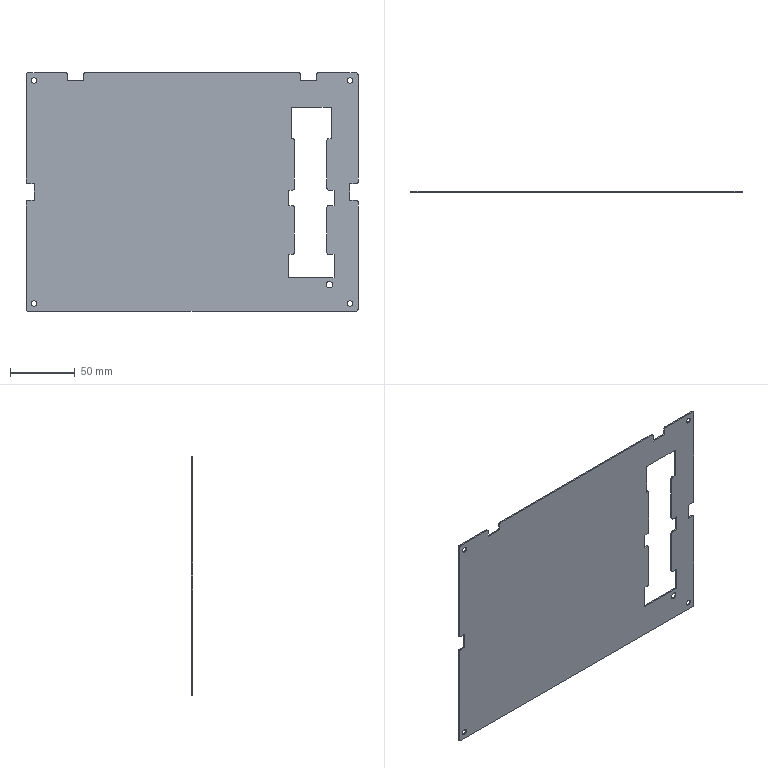Part | SolidWorks | features BaseBody 1 | 1 solid | 74 faces | box 256 x 1 x 184 mm | volume 42983 mm3 | plane 42 | cylinder 32 | commonest cylinder face diameters 3 x20 4.2 x8 2 x2 5 x2